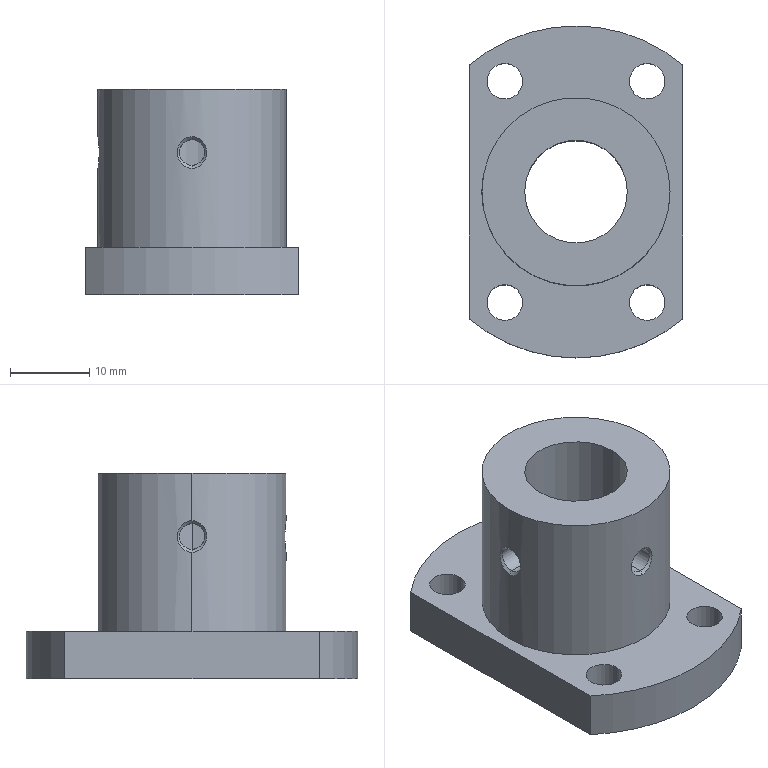Part | STEP file | 001-003-GBC26_D13 | 1 solid | 27 faces | box 27 x 42 x 26 mm | volume 11275 mm3 | cylinder 18 | plane 5 | cone 4 | commonest cylinder face diameters 4.5 x8 3.242 x4 13 x2 23.8 x2 42 x2